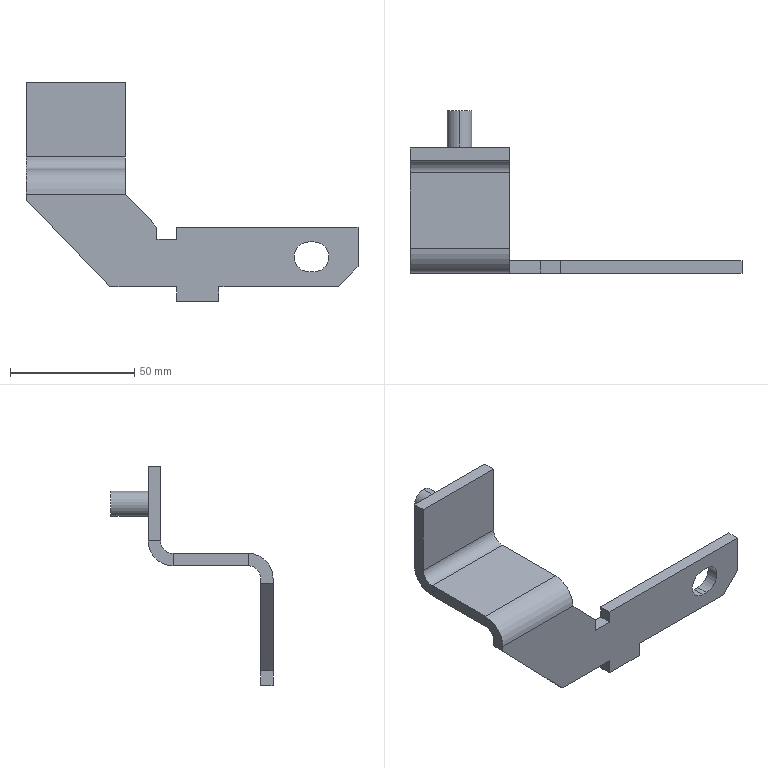Part | STEP file | 64646443 | 1 solid | 42 faces | box 133.75 x 65.3 x 88.252 mm | volume 33570 mm3 | plane 32 | cylinder 10 | commonest cylinder face diameters 10 x4 0.1 x2 12 x2 20 x2